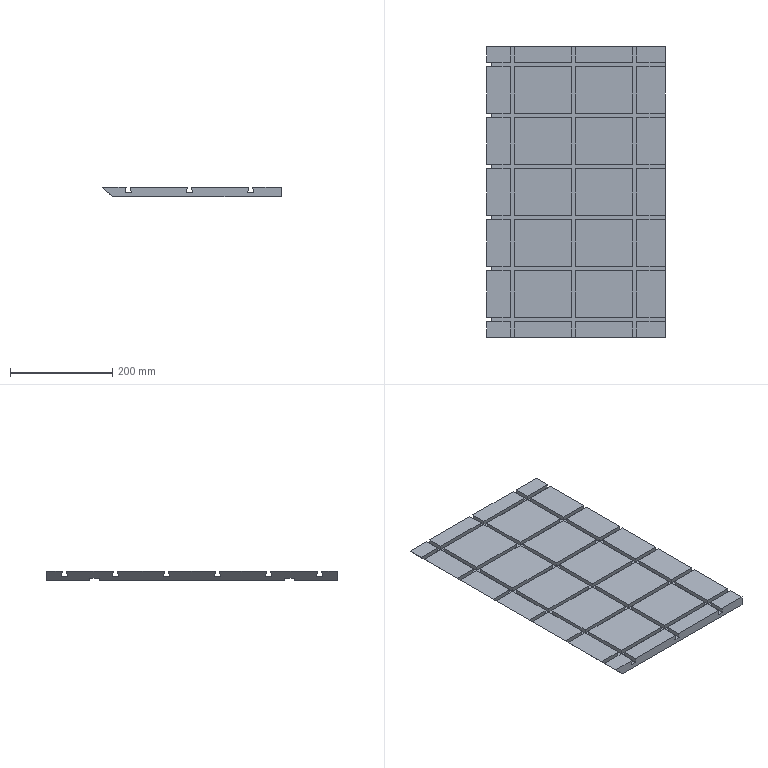Part | STEP file | Superstructure_1 | 1 solid | 132 faces | box 350 x 570 x 19 mm | volume 3268025 mm3 | plane 132